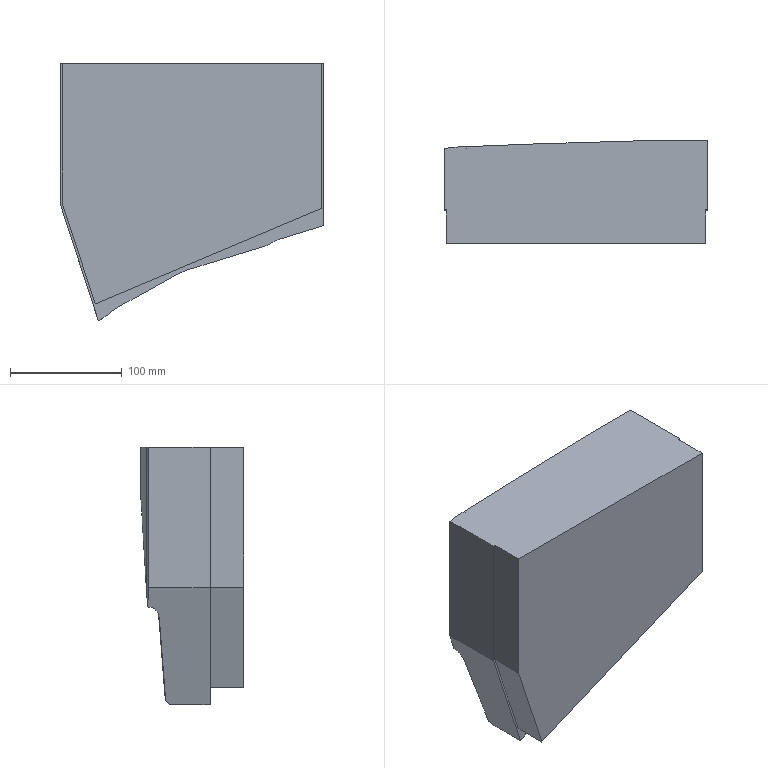Part | NX | features solid 2 | 1 solid | 59 faces | box 236.173 x 92.469 x 230.388 mm | volume 3435174 mm3 | spline 47 | plane 12